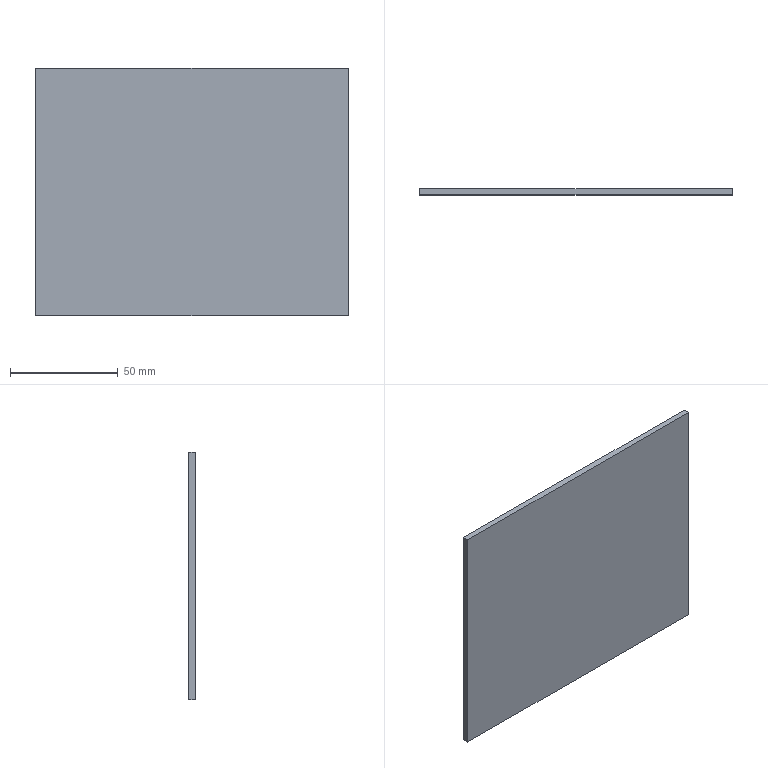Part | Creo | 1 solid | 6 faces | box 145 x 2.8 x 115 mm | volume 46690 mm3 | plane 6
STEP:
#1=CARTESIAN_POINT('',(0.,0.,0.));
#2=DIRECTION('',(0.,0.,1.));
#3=DIRECTION('',(1.,0.,0.));
#4=AXIS2_PLACEMENT_3D('',#1,#2,#3);
#5=CARTESIAN_POINT('',(57.36,4.9,60.));
#6=VERTEX_POINT('',#5);
#7=CARTESIAN_POINT('',(57.36,4.9,-55.));
#8=VERTEX_POINT('',#7);
#9=CARTESIAN_POINT('',(57.36,4.9,60.));
#10=DIRECTION('',(0.,0.,-1.));
#11=VECTOR('',#10,115.);
#12=LINE('',#9,#11);
#13=EDGE_CURVE('',#6,#8,#12,.T.);
#14=ORIENTED_EDGE('',*,*,#13,.T.);
#15=CARTESIAN_POINT('',(-87.64,4.9,-55.));
#16=VERTEX_POINT('',#15);
#17=CARTESIAN_POINT('',(57.36,4.9,-55.));
#18=DIRECTION('',(-1.,0.,0.));
#19=VECTOR('',#18,145.);
#20=LINE('',#17,#19);
#21=EDGE_CURVE('',#8,#16,#20,.T.);
#22=ORIENTED_EDGE('',*,*,#21,.T.);
#23=CARTESIAN_POINT('',(-87.64,4.9,60.));
#24=VERTEX_POINT('',#23);
#25=CARTESIAN_POINT('',(-87.64,4.9,-55.));
#26=DIRECTION('',(0.,0.,1.));
#27=VECTOR('',#26,115.);
#28=LINE('',#25,#27);
#29=EDGE_CURVE('',#16,#24,#28,.T.);
#30=ORIENTED_EDGE('',*,*,#29,.T.);
#31=CARTESIAN_POINT('',(-87.64,4.9,60.));
#32=DIRECTION('',(1.,0.,0.));
#33=VECTOR('',#32,145.);
#34=LINE('',#31,#33);
#35=EDGE_CURVE('',#24,#6,#34,.T.);
#36=ORIENTED_EDGE('',*,*,#35,.T.);
#37=EDGE_LOOP('',(#14,#22,#30,#36));
#38=FACE_OUTER_BOUND('',#37,.F.);
#39=CARTESIAN_POINT('',(0.,4.9,0.));
#40=DIRECTION('',(0.,1.,0.));
#41=DIRECTION('',(-1.,0.,0.));
#42=AXIS2_PLACEMENT_3D('',#39,#40,#41);
#43=PLANE('',#42);
#44=ADVANCED_FACE('',(#38),#43,.F.);
#45=ORIENTED_EDGE('',*,*,#13,.F.);
#46=CARTESIAN_POINT('',(57.36,7.7,60.));
#47=VERTEX_POINT('',#46);
#48=CARTESIAN_POINT('',(57.36,4.9,60.));
#49=DIRECTION('',(0.,1.,0.));
#50=VECTOR('',#49,2.8);
#51=LINE('',#48,#50);
#52=EDGE_CURVE('',#6,#47,#51,.T.);
#53=ORIENTED_EDGE('',*,*,#52,.T.);
#54=CARTESIAN_POINT('',(57.36,7.7,-55.));
#55=VERTEX_POINT('',#54);
#56=CARTESIAN_POINT('',(57.36,7.7,60.));
#57=DIRECTION('',(0.,0.,-1.));
#58=VECTOR('',#57,115.);
#59=LINE('',#56,#58);
#60=EDGE_CURVE('',#47,#55,#59,.T.);
#61=ORIENTED_EDGE('',*,*,#60,.T.);
#62=CARTESIAN_POINT('',(57.36,4.9,-55.));
#63=DIRECTION('',(0.,1.,0.));
#64=VECTOR('',#63,2.8);
#65=LINE('',#62,#64);
#66=EDGE_CURVE('',#8,#55,#65,.T.);
#67=ORIENTED_EDGE('',*,*,#66,.F.);
#68=EDGE_LOOP('',(#45,#53,#61,#67));
#69=FACE_OUTER_BOUND('',#68,.F.);
#70=CARTESIAN_POINT('',(57.36,4.9,60.));
#71=DIRECTION('',(1.,0.,0.));
#72=DIRECTION('',(0.,0.,-1.));
#73=AXIS2_PLACEMENT_3D('',#70,#71,#72);
#74=PLANE('',#73);
#75=ADVANCED_FACE('',(#69),#74,.T.);
#76=ORIENTED_EDGE('',*,*,#35,.F.);
#77=CARTESIAN_POINT('',(-87.64,7.7,60.));
#78=VERTEX_POINT('',#77);
#79=CARTESIAN_POINT('',(-87.64,4.9,60.));
#80=DIRECTION('',(0.,1.,0.));
#81=VECTOR('',#80,2.8);
#82=LINE('',#79,#81);
#83=EDGE_CURVE('',#24,#78,#82,.T.);
#84=ORIENTED_EDGE('',*,*,#83,.T.);
#85=CARTESIAN_POINT('',(-87.64,7.7,60.));
#86=DIRECTION('',(1.,0.,0.));
#87=VECTOR('',#86,145.);
#88=LINE('',#85,#87);
#89=EDGE_CURVE('',#78,#47,#88,.T.);
#90=ORIENTED_EDGE('',*,*,#89,.T.);
#91=ORIENTED_EDGE('',*,*,#52,.F.);
#92=EDGE_LOOP('',(#76,#84,#90,#91));
#93=FACE_OUTER_BOUND('',#92,.F.);
#94=CARTESIAN_POINT('',(-87.64,4.9,60.));
#95=DIRECTION('',(0.,0.,1.));
#96=DIRECTION('',(1.,0.,0.));
#97=AXIS2_PLACEMENT_3D('',#94,#95,#96);
#98=PLANE('',#97);
#99=ADVANCED_FACE('',(#93),#98,.T.);
#100=ORIENTED_EDGE('',*,*,#29,.F.);
#101=CARTESIAN_POINT('',(-87.64,7.7,-55.));
#102=VERTEX_POINT('',#101);
#103=CARTESIAN_POINT('',(-87.64,4.9,-55.));
#104=DIRECTION('',(0.,1.,0.));
#105=VECTOR('',#104,2.8);
#106=LINE('',#103,#105);
#107=EDGE_CURVE('',#16,#102,#106,.T.);
#108=ORIENTED_EDGE('',*,*,#107,.T.);
#109=CARTESIAN_POINT('',(-87.64,7.7,-55.));
#110=DIRECTION('',(0.,0.,1.));
#111=VECTOR('',#110,115.);
#112=LINE('',#109,#111);
#113=EDGE_CURVE('',#102,#78,#112,.T.);
#114=ORIENTED_EDGE('',*,*,#113,.T.);
#115=ORIENTED_EDGE('',*,*,#83,.F.);
#116=EDGE_LOOP('',(#100,#108,#114,#115));
#117=FACE_OUTER_BOUND('',#116,.F.);
#118=CARTESIAN_POINT('',(-87.64,4.9,-55.));
#119=DIRECTION('',(-1.,0.,0.));
#120=DIRECTION('',(0.,0.,1.));
#121=AXIS2_PLACEMENT_3D('',#118,#119,#120);
#122=PLANE('',#121);
#123=ADVANCED_FACE('',(#117),#122,.T.);
#124=ORIENTED_EDGE('',*,*,#21,.F.);
#125=ORIENTED_EDGE('',*,*,#66,.T.);
#126=CARTESIAN_POINT('',(57.36,7.7,-55.));
#127=DIRECTION('',(-1.,0.,0.));
#128=VECTOR('',#127,145.);
#129=LINE('',#126,#128);
#130=EDGE_CURVE('',#55,#102,#129,.T.);
#131=ORIENTED_EDGE('',*,*,#130,.T.);
#132=ORIENTED_EDGE('',*,*,#107,.F.);
#133=EDGE_LOOP('',(#124,#125,#131,#132));
#134=FACE_OUTER_BOUND('',#133,.F.);
#135=CARTESIAN_POINT('',(57.36,4.9,-55.));
#136=DIRECTION('',(0.,0.,-1.));
#137=DIRECTION('',(-1.,0.,0.));
#138=AXIS2_PLACEMENT_3D('',#135,#136,#137);
#139=PLANE('',#138);
#140=ADVANCED_FACE('',(#134),#139,.T.);
#141=ORIENTED_EDGE('',*,*,#60,.F.);
#142=ORIENTED_EDGE('',*,*,#89,.F.);
#143=ORIENTED_EDGE('',*,*,#113,.F.);
#144=ORIENTED_EDGE('',*,*,#130,.F.);
#145=EDGE_LOOP('',(#141,#142,#143,#144));
#146=FACE_OUTER_BOUND('',#145,.F.);
#147=CARTESIAN_POINT('',(0.,7.7,0.));
#148=DIRECTION('',(0.,1.,0.));
#149=DIRECTION('',(-1.,0.,0.));
#150=AXIS2_PLACEMENT_3D('',#147,#148,#149);
#151=PLANE('',#150);
#152=ADVANCED_FACE('',(#146),#151,.T.);
#153=CLOSED_SHELL('',(#44,#75,#99,#123,#140,#152));
#154=MANIFOLD_SOLID_BREP('',#153);
#155=(LENGTH_UNIT()NAMED_UNIT(*)SI_UNIT(.MILLI.,.METRE.));
#156=UNCERTAINTY_MEASURE_WITH_UNIT(LENGTH_MEASURE(0.01851),#155,'','');
#157=(NAMED_UNIT(*)PLANE_ANGLE_UNIT()SI_UNIT($,.RADIAN.));
#158=PLANE_ANGLE_MEASURE_WITH_UNIT(PLANE_ANGLE_MEASURE(0.01745),#157);
#159=(CONVERSION_BASED_UNIT('DEGREE',#158)NAMED_UNIT(*)PLANE_ANGLE_UNIT());
#160=(NAMED_UNIT(*)SI_UNIT($,.STERADIAN.)SOLID_ANGLE_UNIT());
#161=(GEOMETRIC_REPRESENTATION_CONTEXT(3)GLOBAL_UNCERTAINTY_ASSIGNED_CONTEXT((#156))GLOBAL_UNIT_ASSIGNED_CONTEXT((#155,#159,#160))REPRESENTATION_CONTEXT('',''));
#162=ADVANCED_BREP_SHAPE_REPRESENTATION('',(#4,#154),#161);